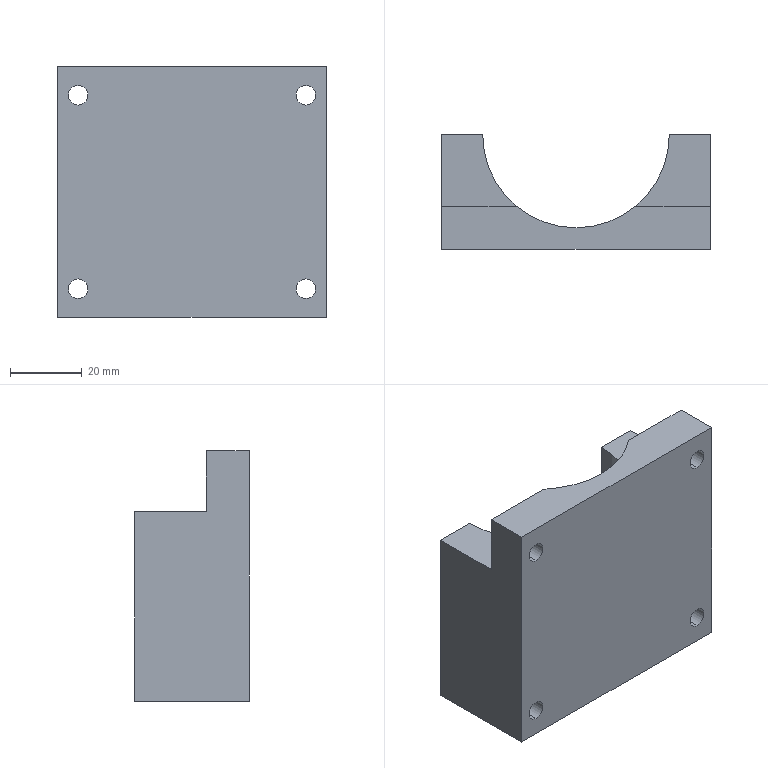Part | SolidWorks | features HoleWzd 2, ICE 2, Extrusion 1 | 1 solid | 48 faces | box 75 x 32 x 70 mm | volume 77130 mm3 | cylinder 25 | plane 15 | cone 8 | commonest cylinder face diameters 4.2 x8 5.5 x8 10 x8 52.1 x1
STEP:
#1=CARTESIAN_POINT('',(-31.75,3.6,18.9));
#2=VERTEX_POINT('',#1);
#3=CARTESIAN_POINT('',(-31.75,3.6,23.1));
#4=VERTEX_POINT('',#3);
#5=CARTESIAN_POINT('',(-31.75,3.6,21.));
#6=DIRECTION('',(0.,1.,0.));
#7=DIRECTION('',(0.,0.,1.));
#8=AXIS2_PLACEMENT_3D('',#5,#6,#7);
#9=CIRCLE('',#8,2.1);
#10=EDGE_CURVE('',#2,#4,#9,.T.);
#11=ORIENTED_EDGE('',*,*,#10,.F.);
#12=CARTESIAN_POINT('',(-31.75,16.,18.9));
#13=VERTEX_POINT('',#12);
#14=CARTESIAN_POINT('',(-31.75,16.,18.9));
#15=DIRECTION('',(0.,1.,0.));
#16=VECTOR('',#15,1000.);
#17=LINE('',#14,#16);
#18=EDGE_CURVE('',#2,#13,#17,.T.);
#19=ORIENTED_EDGE('',*,*,#18,.T.);
#20=CARTESIAN_POINT('',(-31.75,16.,23.1));
#21=VERTEX_POINT('',#20);
#22=CARTESIAN_POINT('',(-31.75,16.,21.));
#23=DIRECTION('',(0.,1.,0.));
#24=DIRECTION('',(0.,0.,1.));
#25=AXIS2_PLACEMENT_3D('',#22,#23,#24);
#26=CIRCLE('',#25,2.1);
#27=EDGE_CURVE('',#13,#21,#26,.T.);
#28=ORIENTED_EDGE('',*,*,#27,.T.);
#29=CARTESIAN_POINT('',(-31.75,16.,23.1));
#30=DIRECTION('',(0.,1.,0.));
#31=VECTOR('',#30,1000.);
#32=LINE('',#29,#31);
#33=EDGE_CURVE('',#4,#21,#32,.T.);
#34=ORIENTED_EDGE('',*,*,#33,.F.);
#35=EDGE_LOOP('',(#11,#19,#28,#34));
#36=FACE_OUTER_BOUND('',#35,.T.);
#37=CARTESIAN_POINT('',(-31.75,16.,21.));
#38=DIRECTION('',(0.,1.,0.));
#39=DIRECTION('',(0.,0.,1.));
#40=AXIS2_PLACEMENT_3D('',#37,#38,#39);
#41=CYLINDRICAL_SURFACE('',#40,2.1);
#42=ADVANCED_FACE('',(#36),#41,.F.);
#43=CARTESIAN_POINT('',(-31.75,2.338,21.));
#44=VERTEX_POINT('',#43);
#45=CARTESIAN_POINT('',(-31.75,3.6,23.1));
#46=DIRECTION('',(0.,0.515,0.8572));
#47=VECTOR('',#46,1000.);
#48=LINE('',#45,#47);
#49=EDGE_CURVE('',#44,#4,#48,.T.);
#50=ORIENTED_EDGE('',*,*,#49,.F.);
#51=CARTESIAN_POINT('',(-31.75,3.6,18.9));
#52=DIRECTION('',(0.,0.515,-0.8572));
#53=VECTOR('',#52,1000.);
#54=LINE('',#51,#53);
#55=EDGE_CURVE('',#44,#2,#54,.T.);
#56=ORIENTED_EDGE('',*,*,#55,.T.);
#57=ORIENTED_EDGE('',*,*,#10,.T.);
#58=EDGE_LOOP('',(#50,#56,#57));
#59=FACE_OUTER_BOUND('',#58,.T.);
#60=CARTESIAN_POINT('',(-31.75,3.6,21.));
#61=DIRECTION('',(0.,1.,0.));
#62=DIRECTION('',(0.,0.,1.));
#63=AXIS2_PLACEMENT_3D('',#60,#61,#62);
#64=CONICAL_SURFACE('',#63,2.1,1.03);
#65=ADVANCED_FACE('',(#59),#64,.F.);
#66=CARTESIAN_POINT('',(-31.75,3.6,42.9));
#67=VERTEX_POINT('',#66);
#68=CARTESIAN_POINT('',(-31.75,3.6,47.1));
#69=VERTEX_POINT('',#68);
#70=CARTESIAN_POINT('',(-31.75,3.6,45.));
#71=DIRECTION('',(0.,1.,0.));
#72=DIRECTION('',(0.,0.,1.));
#73=AXIS2_PLACEMENT_3D('',#70,#71,#72);
#74=CIRCLE('',#73,2.1);
#75=EDGE_CURVE('',#67,#69,#74,.T.);
#76=ORIENTED_EDGE('',*,*,#75,.F.);
#77=CARTESIAN_POINT('',(-31.75,16.,42.9));
#78=VERTEX_POINT('',#77);
#79=CARTESIAN_POINT('',(-31.75,16.,42.9));
#80=DIRECTION('',(0.,1.,0.));
#81=VECTOR('',#80,1000.);
#82=LINE('',#79,#81);
#83=EDGE_CURVE('',#67,#78,#82,.T.);
#84=ORIENTED_EDGE('',*,*,#83,.T.);
#85=CARTESIAN_POINT('',(-31.75,16.,47.1));
#86=VERTEX_POINT('',#85);
#87=CARTESIAN_POINT('',(-31.75,16.,45.));
#88=DIRECTION('',(0.,1.,0.));
#89=DIRECTION('',(0.,0.,1.));
#90=AXIS2_PLACEMENT_3D('',#87,#88,#89);
#91=CIRCLE('',#90,2.1);
#92=EDGE_CURVE('',#78,#86,#91,.T.);
#93=ORIENTED_EDGE('',*,*,#92,.T.);
#94=CARTESIAN_POINT('',(-31.75,16.,47.1));
#95=DIRECTION('',(0.,1.,0.));
#96=VECTOR('',#95,1000.);
#97=LINE('',#94,#96);
#98=EDGE_CURVE('',#69,#86,#97,.T.);
#99=ORIENTED_EDGE('',*,*,#98,.F.);
#100=EDGE_LOOP('',(#76,#84,#93,#99));
#101=FACE_OUTER_BOUND('',#100,.T.);
#102=CARTESIAN_POINT('',(-31.75,16.,45.));
#103=DIRECTION('',(0.,1.,0.));
#104=DIRECTION('',(0.,0.,1.));
#105=AXIS2_PLACEMENT_3D('',#102,#103,#104);
#106=CYLINDRICAL_SURFACE('',#105,2.1);
#107=ADVANCED_FACE('',(#101),#106,.F.);
#108=CARTESIAN_POINT('',(-31.75,2.338,45.));
#109=VERTEX_POINT('',#108);
#110=CARTESIAN_POINT('',(-31.75,3.6,47.1));
#111=DIRECTION('',(0.,0.515,0.8572));
#112=VECTOR('',#111,1000.);
#113=LINE('',#110,#112);
#114=EDGE_CURVE('',#109,#69,#113,.T.);
#115=ORIENTED_EDGE('',*,*,#114,.F.);
#116=CARTESIAN_POINT('',(-31.75,3.6,42.9));
#117=DIRECTION('',(0.,0.515,-0.8572));
#118=VECTOR('',#117,1000.);
#119=LINE('',#116,#118);
#120=EDGE_CURVE('',#109,#67,#119,.T.);
#121=ORIENTED_EDGE('',*,*,#120,.T.);
#122=ORIENTED_EDGE('',*,*,#75,.T.);
#123=EDGE_LOOP('',(#115,#121,#122));
#124=FACE_OUTER_BOUND('',#123,.T.);
#125=CARTESIAN_POINT('',(-31.75,3.6,45.));
#126=DIRECTION('',(0.,1.,0.));
#127=DIRECTION('',(0.,0.,1.));
#128=AXIS2_PLACEMENT_3D('',#125,#126,#127);
#129=CONICAL_SURFACE('',#128,2.1,1.03);
#130=ADVANCED_FACE('',(#124),#129,.F.);
#131=CARTESIAN_POINT('',(31.75,3.6,18.9));
#132=VERTEX_POINT('',#131);
#133=CARTESIAN_POINT('',(31.75,3.6,23.1));
#134=VERTEX_POINT('',#133);
#135=CARTESIAN_POINT('',(31.75,3.6,21.));
#136=DIRECTION('',(0.,1.,0.));
#137=DIRECTION('',(0.,0.,1.));
#138=AXIS2_PLACEMENT_3D('',#135,#136,#137);
#139=CIRCLE('',#138,2.1);
#140=EDGE_CURVE('',#132,#134,#139,.T.);
#141=ORIENTED_EDGE('',*,*,#140,.F.);
#142=CARTESIAN_POINT('',(31.75,16.,18.9));
#143=VERTEX_POINT('',#142);
#144=CARTESIAN_POINT('',(31.75,16.,18.9));
#145=DIRECTION('',(0.,1.,0.));
#146=VECTOR('',#145,1000.);
#147=LINE('',#144,#146);
#148=EDGE_CURVE('',#132,#143,#147,.T.);
#149=ORIENTED_EDGE('',*,*,#148,.T.);
#150=CARTESIAN_POINT('',(31.75,16.,23.1));
#151=VERTEX_POINT('',#150);
#152=CARTESIAN_POINT('',(31.75,16.,21.));
#153=DIRECTION('',(0.,1.,0.));
#154=DIRECTION('',(0.,0.,1.));
#155=AXIS2_PLACEMENT_3D('',#152,#153,#154);
#156=CIRCLE('',#155,2.1);
#157=EDGE_CURVE('',#143,#151,#156,.T.);
#158=ORIENTED_EDGE('',*,*,#157,.T.);
#159=CARTESIAN_POINT('',(31.75,16.,23.1));
#160=DIRECTION('',(0.,1.,0.));
#161=VECTOR('',#160,1000.);
#162=LINE('',#159,#161);
#163=EDGE_CURVE('',#134,#151,#162,.T.);
#164=ORIENTED_EDGE('',*,*,#163,.F.);
#165=EDGE_LOOP('',(#141,#149,#158,#164));
#166=FACE_OUTER_BOUND('',#165,.T.);
#167=CARTESIAN_POINT('',(31.75,16.,21.));
#168=DIRECTION('',(0.,1.,0.));
#169=DIRECTION('',(0.,0.,1.));
#170=AXIS2_PLACEMENT_3D('',#167,#168,#169);
#171=CYLINDRICAL_SURFACE('',#170,2.1);
#172=ADVANCED_FACE('',(#166),#171,.F.);
#173=CARTESIAN_POINT('',(31.75,2.338,21.));
#174=VERTEX_POINT('',#173);
#175=CARTESIAN_POINT('',(31.75,3.6,23.1));
#176=DIRECTION('',(0.,0.515,0.8572));
#177=VECTOR('',#176,1000.);
#178=LINE('',#175,#177);
#179=EDGE_CURVE('',#174,#134,#178,.T.);
#180=ORIENTED_EDGE('',*,*,#179,.F.);
#181=CARTESIAN_POINT('',(31.75,3.6,18.9));
#182=DIRECTION('',(0.,0.515,-0.8572));
#183=VECTOR('',#182,1000.);
#184=LINE('',#181,#183);
#185=EDGE_CURVE('',#174,#132,#184,.T.);
#186=ORIENTED_EDGE('',*,*,#185,.T.);
#187=ORIENTED_EDGE('',*,*,#140,.T.);
#188=EDGE_LOOP('',(#180,#186,#187));
#189=FACE_OUTER_BOUND('',#188,.T.);
#190=CARTESIAN_POINT('',(31.75,3.6,21.));
#191=DIRECTION('',(0.,1.,0.));
#192=DIRECTION('',(0.,0.,1.));
#193=AXIS2_PLACEMENT_3D('',#190,#191,#192);
#194=CONICAL_SURFACE('',#193,2.1,1.03);
#195=ADVANCED_FACE('',(#189),#194,.F.);
#196=CARTESIAN_POINT('',(31.75,3.6,42.9));
#197=VERTEX_POINT('',#196);
#198=CARTESIAN_POINT('',(31.75,3.6,47.1));
#199=VERTEX_POINT('',#198);
#200=CARTESIAN_POINT('',(31.75,3.6,45.));
#201=DIRECTION('',(0.,1.,0.));
#202=DIRECTION('',(0.,0.,1.));
#203=AXIS2_PLACEMENT_3D('',#200,#201,#202);
#204=CIRCLE('',#203,2.1);
#205=EDGE_CURVE('',#197,#199,#204,.T.);
#206=ORIENTED_EDGE('',*,*,#205,.F.);
#207=CARTESIAN_POINT('',(31.75,16.,42.9));
#208=VERTEX_POINT('',#207);
#209=CARTESIAN_POINT('',(31.75,16.,42.9));
#210=DIRECTION('',(0.,1.,0.));
#211=VECTOR('',#210,1000.);
#212=LINE('',#209,#211);
#213=EDGE_CURVE('',#197,#208,#212,.T.);
#214=ORIENTED_EDGE('',*,*,#213,.T.);
#215=CARTESIAN_POINT('',(31.75,16.,47.1));
#216=VERTEX_POINT('',#215);
#217=CARTESIAN_POINT('',(31.75,16.,45.));
#218=DIRECTION('',(0.,1.,0.));
#219=DIRECTION('',(0.,0.,1.));
#220=AXIS2_PLACEMENT_3D('',#217,#218,#219);
#221=CIRCLE('',#220,2.1);
#222=EDGE_CURVE('',#208,#216,#221,.T.);
#223=ORIENTED_EDGE('',*,*,#222,.T.);
#224=CARTESIAN_POINT('',(31.75,16.,47.1));
#225=DIRECTION('',(0.,1.,0.));
#226=VECTOR('',#225,1000.);
#227=LINE('',#224,#226);
#228=EDGE_CURVE('',#199,#216,#227,.T.);
#229=ORIENTED_EDGE('',*,*,#228,.F.);
#230=EDGE_LOOP('',(#206,#214,#223,#229));
#231=FACE_OUTER_BOUND('',#230,.T.);
#232=CARTESIAN_POINT('',(31.75,16.,45.));
#233=DIRECTION('',(0.,1.,0.));
#234=DIRECTION('',(0.,0.,1.));
#235=AXIS2_PLACEMENT_3D('',#232,#233,#234);
#236=CYLINDRICAL_SURFACE('',#235,2.1);
#237=ADVANCED_FACE('',(#231),#236,.F.);
#238=CARTESIAN_POINT('',(31.75,2.338,45.));
#239=VERTEX_POINT('',#238);
#240=CARTESIAN_POINT('',(31.75,3.6,47.1));
#241=DIRECTION('',(0.,0.515,0.8572));
#242=VECTOR('',#241,1000.);
#243=LINE('',#240,#242);
#244=EDGE_CURVE('',#239,#199,#243,.T.);
#245=ORIENTED_EDGE('',*,*,#244,.F.);
#246=CARTESIAN_POINT('',(31.75,3.6,42.9));
#247=DIRECTION('',(0.,0.515,-0.8572));
#248=VECTOR('',#247,1000.);
#249=LINE('',#246,#248);
#250=EDGE_CURVE('',#239,#197,#249,.T.);
#251=ORIENTED_EDGE('',*,*,#250,.T.);
#252=ORIENTED_EDGE('',*,*,#205,.T.);
#253=EDGE_LOOP('',(#245,#251,#252));
#254=FACE_OUTER_BOUND('',#253,.T.);
#255=CARTESIAN_POINT('',(31.75,3.6,45.));
#256=DIRECTION('',(0.,1.,0.));
#257=DIRECTION('',(0.,0.,1.));
#258=AXIS2_PLACEMENT_3D('',#255,#256,#257);
#259=CONICAL_SURFACE('',#258,2.1,1.03);
#260=ADVANCED_FACE('',(#254),#259,.F.);
#261=CARTESIAN_POINT('',(-31.775,-11.,3.));
#262=VERTEX_POINT('',#261);
#263=CARTESIAN_POINT('',(-31.775,-11.,13.));
#264=VERTEX_POINT('',#263);
#265=CARTESIAN_POINT('',(-31.775,-11.,8.));
#266=DIRECTION('',(0.,1.,0.));
#267=DIRECTION('',(0.,0.,1.));
#268=AXIS2_PLACEMENT_3D('',#265,#266,#267);
#269=CIRCLE('',#268,5.);
#270=EDGE_CURVE('',#262,#264,#269,.T.);
#271=ORIENTED_EDGE('',*,*,#270,.F.);
#272=CARTESIAN_POINT('',(-31.775,16.,3.));
#273=VERTEX_POINT('',#272);
#274=CARTESIAN_POINT('',(-31.775,16.,3.));
#275=DIRECTION('',(0.,1.,0.));
#276=VECTOR('',#275,1000.);
#277=LINE('',#274,#276);
#278=EDGE_CURVE('',#262,#273,#277,.T.);
#279=ORIENTED_EDGE('',*,*,#278,.T.);
#280=CARTESIAN_POINT('',(-31.775,16.,13.));
#281=VERTEX_POINT('',#280);
#282=CARTESIAN_POINT('',(-31.775,16.,8.));
#283=DIRECTION('',(0.,1.,0.));
#284=DIRECTION('',(0.,0.,1.));
#285=AXIS2_PLACEMENT_3D('',#282,#283,#284);
#286=CIRCLE('',#285,5.);
#287=EDGE_CURVE('',#273,#281,#286,.T.);
#288=ORIENTED_EDGE('',*,*,#287,.T.);
#289=CARTESIAN_POINT('',(-31.775,16.,13.));
#290=DIRECTION('',(0.,1.,0.));
#291=VECTOR('',#290,1000.);
#292=LINE('',#289,#291);
#293=EDGE_CURVE('',#264,#281,#292,.T.);
#294=ORIENTED_EDGE('',*,*,#293,.F.);
#295=EDGE_LOOP('',(#271,#279,#288,#294));
#296=FACE_OUTER_BOUND('',#295,.T.);
#297=CARTESIAN_POINT('',(-31.775,16.,8.));
#298=DIRECTION('',(0.,1.,0.));
#299=DIRECTION('',(0.,0.,1.));
#300=AXIS2_PLACEMENT_3D('',#297,#298,#299);
#301=CYLINDRICAL_SURFACE('',#300,5.);
#302=ADVANCED_FACE('',(#296),#301,.F.);
#303=CARTESIAN_POINT('',(-31.775,-16.,5.25));
#304=VERTEX_POINT('',#303);
#305=CARTESIAN_POINT('',(-31.775,-16.,10.75));
#306=VERTEX_POINT('',#305);
#307=CARTESIAN_POINT('',(-31.775,-16.,8.));
#308=DIRECTION('',(0.,1.,0.));
#309=DIRECTION('',(0.,0.,1.));
#310=AXIS2_PLACEMENT_3D('',#307,#308,#309);
#311=CIRCLE('',#310,2.75);
#312=EDGE_CURVE('',#304,#306,#311,.T.);
#313=ORIENTED_EDGE('',*,*,#312,.F.);
#314=CARTESIAN_POINT('',(-31.775,-11.,5.25));
#315=VERTEX_POINT('',#314);
#316=CARTESIAN_POINT('',(-31.775,16.,5.25));
#317=DIRECTION('',(0.,1.,0.));
#318=VECTOR('',#317,1000.);
#319=LINE('',#316,#318);
#320=EDGE_CURVE('',#304,#315,#319,.T.);
#321=ORIENTED_EDGE('',*,*,#320,.T.);
#322=CARTESIAN_POINT('',(-31.775,-11.,10.75));
#323=VERTEX_POINT('',#322);
#324=CARTESIAN_POINT('',(-31.775,-11.,8.));
#325=DIRECTION('',(0.,1.,0.));
#326=DIRECTION('',(0.,0.,1.));
#327=AXIS2_PLACEMENT_3D('',#324,#325,#326);
#328=CIRCLE('',#327,2.75);
#329=EDGE_CURVE('',#315,#323,#328,.T.);
#330=ORIENTED_EDGE('',*,*,#329,.T.);
#331=CARTESIAN_POINT('',(-31.775,16.,10.75));
#332=DIRECTION('',(0.,1.,0.));
#333=VECTOR('',#332,1000.);
#334=LINE('',#331,#333);
#335=EDGE_CURVE('',#306,#323,#334,.T.);
#336=ORIENTED_EDGE('',*,*,#335,.F.);
#337=EDGE_LOOP('',(#313,#321,#330,#336));
#338=FACE_OUTER_BOUND('',#337,.T.);
#339=CARTESIAN_POINT('',(-31.775,16.,8.));
#340=DIRECTION('',(0.,1.,0.));
#341=DIRECTION('',(0.,0.,1.));
#342=AXIS2_PLACEMENT_3D('',#339,#340,#341);
#343=CYLINDRICAL_SURFACE('',#342,2.75);
#344=ADVANCED_FACE('',(#338),#343,.F.);
#345=CARTESIAN_POINT('',(-31.775,-11.,57.));
#346=VERTEX_POINT('',#345);
#347=CARTESIAN_POINT('',(-31.775,-11.,67.));
#348=VERTEX_POINT('',#347);
#349=CARTESIAN_POINT('',(-31.775,-11.,62.));
#350=DIRECTION('',(0.,1.,0.));
#351=DIRECTION('',(0.,0.,1.));
#352=AXIS2_PLACEMENT_3D('',#349,#350,#351);
#353=CIRCLE('',#352,5.);
#354=EDGE_CURVE('',#346,#348,#353,.T.);
#355=ORIENTED_EDGE('',*,*,#354,.F.);
#356=CARTESIAN_POINT('',(-31.775,-4.,57.));
#357=VERTEX_POINT('',#356);
#358=CARTESIAN_POINT('',(-31.775,16.,57.));
#359=DIRECTION('',(0.,1.,0.));
#360=VECTOR('',#359,1000.);
#361=LINE('',#358,#360);
#362=EDGE_CURVE('',#346,#357,#361,.T.);
#363=ORIENTED_EDGE('',*,*,#362,.T.);
#364=CARTESIAN_POINT('',(-31.775,-4.,67.));
#365=VERTEX_POINT('',#364);
#366=CARTESIAN_POINT('',(-31.775,-4.,62.));
#367=DIRECTION('',(0.,1.,0.));
#368=DIRECTION('',(0.,0.,-1.));
#369=AXIS2_PLACEMENT_3D('',#366,#367,#368);
#370=CIRCLE('',#369,5.);
#371=EDGE_CURVE('',#357,#365,#370,.T.);
#372=ORIENTED_EDGE('',*,*,#371,.T.);
#373=CARTESIAN_POINT('',(-31.775,16.,67.));
#374=DIRECTION('',(0.,1.,0.));
#375=VECTOR('',#374,1000.);
#376=LINE('',#373,#375);
#377=EDGE_CURVE('',#348,#365,#376,.T.);
#378=ORIENTED_EDGE('',*,*,#377,.F.);
#379=EDGE_LOOP('',(#355,#363,#372,#378));
#380=FACE_OUTER_BOUND('',#379,.T.);
#381=CARTESIAN_POINT('',(-31.775,16.,62.));
#382=DIRECTION('',(0.,1.,0.));
#383=DIRECTION('',(0.,0.,1.));
#384=AXIS2_PLACEMENT_3D('',#381,#382,#383);
#385=CYLINDRICAL_SURFACE('',#384,5.);
#386=ADVANCED_FACE('',(#380),#385,.F.);
#387=CARTESIAN_POINT('',(-31.775,-16.,59.25));
#388=VERTEX_POINT('',#387);
#389=CARTESIAN_POINT('',(-31.775,-16.,64.75));
#390=VERTEX_POINT('',#389);
#391=CARTESIAN_POINT('',(-31.775,-16.,62.));
#392=DIRECTION('',(0.,1.,0.));
#393=DIRECTION('',(0.,0.,1.));
#394=AXIS2_PLACEMENT_3D('',#391,#392,#393);
#395=CIRCLE('',#394,2.75);
#396=EDGE_CURVE('',#388,#390,#395,.T.);
#397=ORIENTED_EDGE('',*,*,#396,.F.);
#398=CARTESIAN_POINT('',(-31.775,-11.,59.25));
#399=VERTEX_POINT('',#398);
#400=CARTESIAN_POINT('',(-31.775,16.,59.25));
#401=DIRECTION('',(0.,1.,0.));
#402=VECTOR('',#401,1000.);
#403=LINE('',#400,#402);
#404=EDGE_CURVE('',#388,#399,#403,.T.);
#405=ORIENTED_EDGE('',*,*,#404,.T.);
#406=CARTESIAN_POINT('',(-31.775,-11.,64.75));
#407=VERTEX_POINT('',#406);
#408=CARTESIAN_POINT('',(-31.775,-11.,62.));
#409=DIRECTION('',(0.,1.,0.));
#410=DIRECTION('',(0.,0.,1.));
#411=AXIS2_PLACEMENT_3D('',#408,#409,#410);
#412=CIRCLE('',#411,2.75);
#413=EDGE_CURVE('',#399,#407,#412,.T.);
#414=ORIENTED_EDGE('',*,*,#413,.T.);
#415=CARTESIAN_POINT('',(-31.775,16.,64.75));
#416=DIRECTION('',(0.,1.,0.));
#417=VECTOR('',#416,1000.);
#418=LINE('',#415,#417);
#419=EDGE_CURVE('',#390,#407,#418,.T.);
#420=ORIENTED_EDGE('',*,*,#419,.F.);
#421=EDGE_LOOP('',(#397,#405,#414,#420));
#422=FACE_OUTER_BOUND('',#421,.T.);
#423=CARTESIAN_POINT('',(-31.775,16.,62.));
#424=DIRECTION('',(0.,1.,0.));
#425=DIRECTION('',(0.,0.,1.));
#426=AXIS2_PLACEMENT_3D('',#423,#424,#425);
#427=CYLINDRICAL_SURFACE('',#426,2.75);
#428=ADVANCED_FACE('',(#422),#427,.F.);
#429=CARTESIAN_POINT('',(31.775,-11.,57.));
#430=VERTEX_POINT('',#429);
#431=CARTESIAN_POINT('',(31.775,-11.,67.));
#432=VERTEX_POINT('',#431);
#433=CARTESIAN_POINT('',(31.775,-11.,62.));
#434=DIRECTION('',(0.,1.,0.));
#435=DIRECTION('',(0.,0.,1.));
#436=AXIS2_PLACEMENT_3D('',#433,#434,#435);
#437=CIRCLE('',#436,5.);
#438=EDGE_CURVE('',#430,#432,#437,.T.);
#439=ORIENTED_EDGE('',*,*,#438,.F.);
#440=CARTESIAN_POINT('',(31.775,-4.,57.));
#441=VERTEX_POINT('',#440);
#442=CARTESIAN_POINT('',(31.775,16.,57.));
#443=DIRECTION('',(0.,1.,0.));
#444=VECTOR('',#443,1000.);
#445=LINE('',#442,#444);
#446=EDGE_CURVE('',#430,#441,#445,.T.);
#447=ORIENTED_EDGE('',*,*,#446,.T.);
#448=CARTESIAN_POINT('',(31.775,-4.,67.));
#449=VERTEX_POINT('',#448);
#450=CARTESIAN_POINT('',(31.775,-4.,62.));
#451=DIRECTION('',(0.,1.,0.));
#452=DIRECTION('',(0.,0.,-1.));
#453=AXIS2_PLACEMENT_3D('',#450,#451,#452);
#454=CIRCLE('',#453,5.);
#455=EDGE_CURVE('',#441,#449,#454,.T.);
#456=ORIENTED_EDGE('',*,*,#455,.T.);
#457=CARTESIAN_POINT('',(31.775,16.,67.));
#458=DIRECTION('',(0.,1.,0.));
#459=VECTOR('',#458,1000.);
#460=LINE('',#457,#459);
#461=EDGE_CURVE('',#432,#449,#460,.T.);
#462=ORIENTED_EDGE('',*,*,#461,.F.);
#463=EDGE_LOOP('',(#439,#447,#456,#462));
#464=FACE_OUTER_BOUND('',#463,.T.);
#465=CARTESIAN_POINT('',(31.775,16.,62.));
#466=DIRECTION('',(0.,1.,0.));
#467=DIRECTION('',(0.,0.,1.));
#468=AXIS2_PLACEMENT_3D('',#465,#466,#467);
#469=CYLINDRICAL_SURFACE('',#468,5.);
#470=ADVANCED_FACE('',(#464),#469,.F.);
#471=CARTESIAN_POINT('',(31.775,-16.,59.25));
#472=VERTEX_POINT('',#471);
#473=CARTESIAN_POINT('',(31.775,-16.,64.75));
#474=VERTEX_POINT('',#473);
#475=CARTESIAN_POINT('',(31.775,-16.,62.));
#476=DIRECTION('',(0.,1.,0.));
#477=DIRECTION('',(0.,0.,1.));
#478=AXIS2_PLACEMENT_3D('',#475,#476,#477);
#479=CIRCLE('',#478,2.75);
#480=EDGE_CURVE('',#472,#474,#479,.T.);
#481=ORIENTED_EDGE('',*,*,#480,.F.);
#482=CARTESIAN_POINT('',(31.775,-11.,59.25));
#483=VERTEX_POINT('',#482);
#484=CARTESIAN_POINT('',(31.775,16.,59.25));
#485=DIRECTION('',(0.,1.,0.));
#486=VECTOR('',#485,1000.);
#487=LINE('',#484,#486);
#488=EDGE_CURVE('',#472,#483,#487,.T.);
#489=ORIENTED_EDGE('',*,*,#488,.T.);
#490=CARTESIAN_POINT('',(31.775,-11.,64.75));
#491=VERTEX_POINT('',#490);
#492=CARTESIAN_POINT('',(31.775,-11.,62.));
#493=DIRECTION('',(0.,1.,0.));
#494=DIRECTION('',(0.,0.,1.));
#495=AXIS2_PLACEMENT_3D('',#492,#493,#494);
#496=CIRCLE('',#495,2.75);
#497=EDGE_CURVE('',#483,#491,#496,.T.);
#498=ORIENTED_EDGE('',*,*,#497,.T.);
#499=CARTESIAN_POINT('',(31.775,16.,64.75));
#500=DIRECTION('',(0.,1.,0.));
#501=VECTOR('',#500,1000.);
#502=LINE('',#499,#501);
#503=EDGE_CURVE('',#474,#491,#502,.T.);
#504=ORIENTED_EDGE('',*,*,#503,.F.);
#505=EDGE_LOOP('',(#481,#489,#498,#504));
#506=FACE_OUTER_BOUND('',#505,.T.);
#507=CARTESIAN_POINT('',(31.775,16.,62.));
#508=DIRECTION('',(0.,1.,0.));
#509=DIRECTION('',(0.,0.,1.));
#510=AXIS2_PLACEMENT_3D('',#507,#508,#509);
#511=CYLINDRICAL_SURFACE('',#510,2.75);
#512=ADVANCED_FACE('',(#506),#511,.F.);
#513=CARTESIAN_POINT('',(31.775,-11.,3.));
#514=VERTEX_POINT('',#513);
#515=CARTESIAN_POINT('',(31.775,-11.,13.));
#516=VERTEX_POINT('',#515);
#517=CARTESIAN_POINT('',(31.775,-11.,8.));
#518=DIRECTION('',(0.,1.,0.));
#519=DIRECTION('',(0.,0.,1.));
#520=AXIS2_PLACEMENT_3D('',#517,#518,#519);
#521=CIRCLE('',#520,5.);
#522=EDGE_CURVE('',#514,#516,#521,.T.);
#523=ORIENTED_EDGE('',*,*,#522,.F.);
#524=CARTESIAN_POINT('',(31.775,16.,3.));
#525=VERTEX_POINT('',#524);
#526=CARTESIAN_POINT('',(31.775,16.,3.));
#527=DIRECTION('',(0.,1.,0.));
#528=VECTOR('',#527,1000.);
#529=LINE('',#526,#528);
#530=EDGE_CURVE('',#514,#525,#529,.T.);
#531=ORIENTED_EDGE('',*,*,#530,.T.);
#532=CARTESIAN_POINT('',(31.775,16.,13.));
#533=VERTEX_POINT('',#532);
#534=CARTESIAN_POINT('',(31.775,16.,8.));
#535=DIRECTION('',(0.,1.,0.));
#536=DIRECTION('',(0.,0.,1.));
#537=AXIS2_PLACEMENT_3D('',#534,#535,#536);
#538=CIRCLE('',#537,5.);
#539=EDGE_CURVE('',#525,#533,#538,.T.);
#540=ORIENTED_EDGE('',*,*,#539,.T.);
#541=CARTESIAN_POINT('',(31.775,16.,13.));
#542=DIRECTION('',(0.,1.,0.));
#543=VECTOR('',#542,1000.);
#544=LINE('',#541,#543);
#545=EDGE_CURVE('',#516,#533,#544,.T.);
#546=ORIENTED_EDGE('',*,*,#545,.F.);
#547=EDGE_LOOP('',(#523,#531,#540,#546));
#548=FACE_OUTER_BOUND('',#547,.T.);
#549=CARTESIAN_POINT('',(31.775,16.,8.));
#550=DIRECTION('',(0.,1.,0.));
#551=DIRECTION('',(0.,0.,1.));
#552=AXIS2_PLACEMENT_3D('',#549,#550,#551);
#553=CYLINDRICAL_SURFACE('',#552,5.);
#554=ADVANCED_FACE('',(#548),#553,.F.);
#555=CARTESIAN_POINT('',(31.775,-16.,5.25));
#556=VERTEX_POINT('',#555);
#557=CARTESIAN_POINT('',(31.775,-16.,10.75));
#558=VERTEX_POINT('',#557);
#559=CARTESIAN_POINT('',(31.775,-16.,8.));
#560=DIRECTION('',(0.,1.,0.));
#561=DIRECTION('',(0.,0.,1.));
#562=AXIS2_PLACEMENT_3D('',#559,#560,#561);
#563=CIRCLE('',#562,2.75);
#564=EDGE_CURVE('',#556,#558,#563,.T.);
#565=ORIENTED_EDGE('',*,*,#564,.F.);
#566=CARTESIAN_POINT('',(31.775,-11.,5.25));
#567=VERTEX_POINT('',#566);
#568=CARTESIAN_POINT('',(31.775,16.,5.25));
#569=DIRECTION('',(0.,1.,0.));
#570=VECTOR('',#569,1000.);
#571=LINE('',#568,#570);
#572=EDGE_CURVE('',#556,#567,#571,.T.);
#573=ORIENTED_EDGE('',*,*,#572,.T.);
#574=CARTESIAN_POINT('',(31.775,-11.,10.75));
#575=VERTEX_POINT('',#574);
#576=CARTESIAN_POINT('',(31.775,-11.,8.));
#577=DIRECTION('',(0.,1.,0.));
#578=DIRECTION('',(0.,0.,1.));
#579=AXIS2_PLACEMENT_3D('',#576,#577,#578);
#580=CIRCLE('',#579,2.75);
#581=EDGE_CURVE('',#567,#575,#580,.T.);
#582=ORIENTED_EDGE('',*,*,#581,.T.);
#583=CARTESIAN_POINT('',(31.775,16.,10.75));
#584=DIRECTION('',(0.,1.,0.));
#585=VECTOR('',#584,1000.);
#586=LINE('',#583,#585);
#587=EDGE_CURVE('',#558,#575,#586,.T.);
#588=ORIENTED_EDGE('',*,*,#587,.F.);
#589=EDGE_LOOP('',(#565,#573,#582,#588));
#590=FACE_OUTER_BOUND('',#589,.T.);
#591=CARTESIAN_POINT('',(31.775,16.,8.));
#592=DIRECTION('',(0.,1.,0.));
#593=DIRECTION('',(0.,0.,1.));
#594=AXIS2_PLACEMENT_3D('',#591,#592,#593);
#595=CYLINDRICAL_SURFACE('',#594,2.75);
#596=ADVANCED_FACE('',(#590),#595,.F.);
#597=CARTESIAN_POINT('',(31.75,16.,21.));
#598=DIRECTION('',(0.,1.,0.));
#599=DIRECTION('',(0.,0.,1.));
#600=AXIS2_PLACEMENT_3D('',#597,#598,#599);
#601=CIRCLE('',#600,2.1);
#602=EDGE_CURVE('',#151,#143,#601,.T.);
#603=ORIENTED_EDGE('',*,*,#602,.F.);
#604=ORIENTED_EDGE('',*,*,#157,.F.);
#605=EDGE_LOOP('',(#603,#604));
#606=FACE_BOUND('',#605,.T.);
#607=CARTESIAN_POINT('',(31.75,16.,45.));
#608=DIRECTION('',(0.,1.,0.));
#609=DIRECTION('',(0.,0.,1.));
#610=AXIS2_PLACEMENT_3D('',#607,#608,#609);
#611=CIRCLE('',#610,2.1);
#612=EDGE_CURVE('',#216,#208,#611,.T.);
#613=ORIENTED_EDGE('',*,*,#612,.F.);
#614=ORIENTED_EDGE('',*,*,#222,.F.);
#615=EDGE_LOOP('',(#613,#614));
#616=FACE_BOUND('',#615,.T.);
#617=CARTESIAN_POINT('',(31.775,16.,8.));
#618=DIRECTION('',(0.,1.,0.));
#619=DIRECTION('',(0.,0.,1.));
#620=AXIS2_PLACEMENT_3D('',#617,#618,#619);
#621=CIRCLE('',#620,5.);
#622=EDGE_CURVE('',#533,#525,#621,.T.);
#623=ORIENTED_EDGE('',*,*,#622,.F.);
#624=ORIENTED_EDGE('',*,*,#539,.F.);
#625=EDGE_LOOP('',(#623,#624));
#626=FACE_BOUND('',#625,.T.);
#627=CARTESIAN_POINT('',(26.05,16.,0.));
#628=VERTEX_POINT('',#627);
#629=CARTESIAN_POINT('',(26.05,16.,53.));
#630=VERTEX_POINT('',#629);
#631=CARTESIAN_POINT('',(26.05,16.,0.));
#632=DIRECTION('',(0.,0.,1.));
#633=VECTOR('',#632,1000.);
#634=LINE('',#631,#633);
#635=EDGE_CURVE('',#628,#630,#634,.T.);
#636=ORIENTED_EDGE('',*,*,#635,.T.);
#637=CARTESIAN_POINT('',(37.5,16.,53.));
#638=VERTEX_POINT('',#637);
#639=CARTESIAN_POINT('',(37.5,16.,53.));
#640=DIRECTION('',(-1.,0.,0.));
#641=VECTOR('',#640,1000.);
#642=LINE('',#639,#641);
#643=EDGE_CURVE('',#638,#630,#642,.T.);
#644=ORIENTED_EDGE('',*,*,#643,.F.);
#645=CARTESIAN_POINT('',(37.5,16.,0.));
#646=VERTEX_POINT('',#645);
#647=CARTESIAN_POINT('',(37.5,16.,70.));
#648=DIRECTION('',(0.,0.,-1.));
#649=VECTOR('',#648,1000.);
#650=LINE('',#647,#649);
#651=EDGE_CURVE('',#638,#646,#650,.T.);
#652=ORIENTED_EDGE('',*,*,#651,.T.);
#653=CARTESIAN_POINT('',(-37.5,16.,0.));
#654=DIRECTION('',(-1.,0.,0.));
#655=VECTOR('',#654,1000.);
#656=LINE('',#653,#655);
#657=EDGE_CURVE('',#646,#628,#656,.T.);
#658=ORIENTED_EDGE('',*,*,#657,.T.);
#659=EDGE_LOOP('',(#636,#644,#652,#658));
#660=FACE_OUTER_BOUND('',#659,.T.);
#661=CARTESIAN_POINT('',(-37.5,16.,70.));
#662=DIRECTION('',(0.,-1.,0.));
#663=DIRECTION('',(0.,0.,-1.));
#664=AXIS2_PLACEMENT_3D('',#661,#662,#663);
#665=PLANE('',#664);
#666=ADVANCED_FACE('',(#606,#616,#626,#660),#665,.F.);
#667=ORIENTED_EDGE('',*,*,#651,.F.);
#668=CARTESIAN_POINT('',(37.5,-4.,53.));
#669=VERTEX_POINT('',#668);
#670=CARTESIAN_POINT('',(37.5,16.,53.));
#671=DIRECTION('',(0.,-1.,0.));
#672=VECTOR('',#671,1000.);
#673=LINE('',#670,#672);
#674=EDGE_CURVE('',#638,#669,#673,.T.);
#675=ORIENTED_EDGE('',*,*,#674,.T.);
#676=CARTESIAN_POINT('',(37.5,-4.,70.));
#677=VERTEX_POINT('',#676);
#678=CARTESIAN_POINT('',(37.5,-4.,53.));
#679=DIRECTION('',(0.,0.,1.));
#680=VECTOR('',#679,1000.);
#681=LINE('',#678,#680);
#682=EDGE_CURVE('',#669,#677,#681,.T.);
#683=ORIENTED_EDGE('',*,*,#682,.T.);
#684=CARTESIAN_POINT('',(37.5,-16.,70.));
#685=VERTEX_POINT('',#684);
#686=CARTESIAN_POINT('',(37.5,-16.,70.));
#687=DIRECTION('',(0.,1.,0.));
#688=VECTOR('',#687,1000.);
#689=LINE('',#686,#688);
#690=EDGE_CURVE('',#685,#677,#689,.T.);
#691=ORIENTED_EDGE('',*,*,#690,.F.);
#692=CARTESIAN_POINT('',(37.5,-16.,0.));
#693=VERTEX_POINT('',#692);
#694=CARTESIAN_POINT('',(37.5,-16.,70.));
#695=DIRECTION('',(0.,0.,-1.));
#696=VECTOR('',#695,1000.);
#697=LINE('',#694,#696);
#698=EDGE_CURVE('',#685,#693,#697,.T.);
#699=ORIENTED_EDGE('',*,*,#698,.T.);
#700=CARTESIAN_POINT('',(37.5,-16.,0.));
#701=DIRECTION('',(0.,1.,0.));
#702=VECTOR('',#701,1000.);
#703=LINE('',#700,#702);
#704=EDGE_CURVE('',#693,#646,#703,.T.);
#705=ORIENTED_EDGE('',*,*,#704,.T.);
#706=EDGE_LOOP('',(#667,#675,#683,#691,#699,#705));
#707=FACE_OUTER_BOUND('',#706,.T.);
#708=CARTESIAN_POINT('',(37.5,-16.,70.));
#709=DIRECTION('',(-1.,0.,0.));
#710=DIRECTION('',(0.,0.,1.));
#711=AXIS2_PLACEMENT_3D('',#708,#709,#710);
#712=PLANE('',#711);
#713=ADVANCED_FACE('',(#707),#712,.F.);
#714=CARTESIAN_POINT('',(-31.75,16.,21.));
#715=DIRECTION('',(0.,1.,0.));
#716=DIRECTION('',(0.,0.,1.));
#717=AXIS2_PLACEMENT_3D('',#714,#715,#716);
#718=CIRCLE('',#717,2.1);
#719=EDGE_CURVE('',#21,#13,#718,.T.);
#720=ORIENTED_EDGE('',*,*,#719,.F.);
#721=ORIENTED_EDGE('',*,*,#27,.F.);
#722=EDGE_LOOP('',(#720,#721));
#723=FACE_BOUND('',#722,.T.);
#724=CARTESIAN_POINT('',(-31.75,16.,45.));
#725=DIRECTION('',(0.,1.,0.));
#726=DIRECTION('',(0.,0.,1.));
#727=AXIS2_PLACEMENT_3D('',#724,#725,#726);
#728=CIRCLE('',#727,2.1);
#729=EDGE_CURVE('',#86,#78,#728,.T.);
#730=ORIENTED_EDGE('',*,*,#729,.F.);
#731=ORIENTED_EDGE('',*,*,#92,.F.);
#732=EDGE_LOOP('',(#730,#731));
#733=FACE_BOUND('',#732,.T.);
#734=CARTESIAN_POINT('',(-31.775,16.,8.));
#735=DIRECTION('',(0.,1.,0.));
#736=DIRECTION('',(0.,0.,1.));
#737=AXIS2_PLACEMENT_3D('',#734,#735,#736);
#738=CIRCLE('',#737,5.);
#739=EDGE_CURVE('',#281,#273,#738,.T.);
#740=ORIENTED_EDGE('',*,*,#739,.F.);
#741=ORIENTED_EDGE('',*,*,#287,.F.);
#742=EDGE_LOOP('',(#740,#741));
#743=FACE_BOUND('',#742,.T.);
#744=CARTESIAN_POINT('',(-37.5,16.,53.));
#745=VERTEX_POINT('',#744);
#746=CARTESIAN_POINT('',(-37.5,16.,0.));
#747=VERTEX_POINT('',#746);
#748=CARTESIAN_POINT('',(-37.5,16.,70.));
#749=DIRECTION('',(0.,0.,-1.));
#750=VECTOR('',#749,1000.);
#751=LINE('',#748,#750);
#752=EDGE_CURVE('',#745,#747,#751,.T.);
#753=ORIENTED_EDGE('',*,*,#752,.F.);
#754=CARTESIAN_POINT('',(-26.05,16.,53.));
#755=VERTEX_POINT('',#754);
#756=CARTESIAN_POINT('',(37.5,16.,53.));
#757=DIRECTION('',(-1.,0.,0.));
#758=VECTOR('',#757,1000.);
#759=LINE('',#756,#758);
#760=EDGE_CURVE('',#755,#745,#759,.T.);
#761=ORIENTED_EDGE('',*,*,#760,.F.);
#762=CARTESIAN_POINT('',(-26.05,16.,0.));
#763=VERTEX_POINT('',#762);
#764=CARTESIAN_POINT('',(-26.05,16.,0.));
#765=DIRECTION('',(0.,0.,-1.));
#766=VECTOR('',#765,1000.);
#767=LINE('',#764,#766);
#768=EDGE_CURVE('',#755,#763,#767,.T.);
#769=ORIENTED_EDGE('',*,*,#768,.T.);
#770=CARTESIAN_POINT('',(-37.5,16.,0.));
#771=DIRECTION('',(-1.,0.,0.));
#772=VECTOR('',#771,1000.);
#773=LINE('',#770,#772);
#774=EDGE_CURVE('',#763,#747,#773,.T.);
#775=ORIENTED_EDGE('',*,*,#774,.T.);
#776=EDGE_LOOP('',(#753,#761,#769,#775));
#777=FACE_OUTER_BOUND('',#776,.T.);
#778=CARTESIAN_POINT('',(-37.5,16.,70.));
#779=DIRECTION('',(0.,-1.,0.));
#780=DIRECTION('',(0.,0.,-1.));
#781=AXIS2_PLACEMENT_3D('',#778,#779,#780);
#782=PLANE('',#781);
#783=ADVANCED_FACE('',(#723,#733,#743,#777),#782,.F.);
#784=CARTESIAN_POINT('',(-37.5,-4.,53.));
#785=VERTEX_POINT('',#784);
#786=CARTESIAN_POINT('',(-37.5,-4.,70.));
#787=VERTEX_POINT('',#786);
#788=CARTESIAN_POINT('',(-37.5,-4.,53.));
#789=DIRECTION('',(0.,0.,1.));
#790=VECTOR('',#789,1000.);
#791=LINE('',#788,#790);
#792=EDGE_CURVE('',#785,#787,#791,.T.);
#793=ORIENTED_EDGE('',*,*,#792,.F.);
#794=CARTESIAN_POINT('',(-37.5,16.,53.));
#795=DIRECTION('',(0.,-1.,0.));
#796=VECTOR('',#795,1000.);
#797=LINE('',#794,#796);
#798=EDGE_CURVE('',#745,#785,#797,.T.);
#799=ORIENTED_EDGE('',*,*,#798,.F.);
#800=ORIENTED_EDGE('',*,*,#752,.T.);
#801=CARTESIAN_POINT('',(-37.5,-16.,0.));
#802=VERTEX_POINT('',#801);
#803=CARTESIAN_POINT('',(-37.5,-16.,0.));
#804=DIRECTION('',(0.,-1.,0.));
#805=VECTOR('',#804,1000.);
#806=LINE('',#803,#805);
#807=EDGE_CURVE('',#747,#802,#806,.T.);
#808=ORIENTED_EDGE('',*,*,#807,.T.);
#809=CARTESIAN_POINT('',(-37.5,-16.,70.));
#810=VERTEX_POINT('',#809);
#811=CARTESIAN_POINT('',(-37.5,-16.,70.));
#812=DIRECTION('',(0.,0.,-1.));
#813=VECTOR('',#812,1000.);
#814=LINE('',#811,#813);
#815=EDGE_CURVE('',#810,#802,#814,.T.);
#816=ORIENTED_EDGE('',*,*,#815,.F.);
#817=CARTESIAN_POINT('',(-37.5,-16.,70.));
#818=DIRECTION('',(0.,-1.,0.));
#819=VECTOR('',#818,1000.);
#820=LINE('',#817,#819);
#821=EDGE_CURVE('',#787,#810,#820,.T.);
#822=ORIENTED_EDGE('',*,*,#821,.F.);
#823=EDGE_LOOP('',(#793,#799,#800,#808,#816,#822));
#824=FACE_OUTER_BOUND('',#823,.T.);
#825=CARTESIAN_POINT('',(-37.5,-16.,70.));
#826=DIRECTION('',(1.,0.,0.));
#827=DIRECTION('',(0.,0.,-1.));
#828=AXIS2_PLACEMENT_3D('',#825,#826,#827);
#829=PLANE('',#828);
#830=ADVANCED_FACE('',(#824),#829,.F.);
#831=CARTESIAN_POINT('',(-31.775,-16.,8.));
#832=DIRECTION('',(0.,1.,0.));
#833=DIRECTION('',(0.,0.,1.));
#834=AXIS2_PLACEMENT_3D('',#831,#832,#833);
#835=CIRCLE('',#834,2.75);
#836=EDGE_CURVE('',#306,#304,#835,.T.);
#837=ORIENTED_EDGE('',*,*,#836,.T.);
#838=ORIENTED_EDGE('',*,*,#312,.T.);
#839=EDGE_LOOP('',(#837,#838));
#840=FACE_BOUND('',#839,.T.);
#841=CARTESIAN_POINT('',(-31.775,-16.,62.));
#842=DIRECTION('',(0.,1.,0.));
#843=DIRECTION('',(0.,0.,1.));
#844=AXIS2_PLACEMENT_3D('',#841,#842,#843);
#845=CIRCLE('',#844,2.75);
#846=EDGE_CURVE('',#390,#388,#845,.T.);
#847=ORIENTED_EDGE('',*,*,#846,.T.);
#848=ORIENTED_EDGE('',*,*,#396,.T.);
#849=EDGE_LOOP('',(#847,#848));
#850=FACE_BOUND('',#849,.T.);
#851=CARTESIAN_POINT('',(31.775,-16.,62.));
#852=DIRECTION('',(0.,1.,0.));
#853=DIRECTION('',(0.,0.,1.));
#854=AXIS2_PLACEMENT_3D('',#851,#852,#853);
#855=CIRCLE('',#854,2.75);
#856=EDGE_CURVE('',#474,#472,#855,.T.);
#857=ORIENTED_EDGE('',*,*,#856,.T.);
#858=ORIENTED_EDGE('',*,*,#480,.T.);
#859=EDGE_LOOP('',(#857,#858));
#860=FACE_BOUND('',#859,.T.);
#861=CARTESIAN_POINT('',(31.775,-16.,8.));
#862=DIRECTION('',(0.,1.,0.));
#863=DIRECTION('',(0.,0.,1.));
#864=AXIS2_PLACEMENT_3D('',#861,#862,#863);
#865=CIRCLE('',#864,2.75);
#866=EDGE_CURVE('',#558,#556,#865,.T.);
#867=ORIENTED_EDGE('',*,*,#866,.T.);
#868=ORIENTED_EDGE('',*,*,#564,.T.);
#869=EDGE_LOOP('',(#867,#868));
#870=FACE_BOUND('',#869,.T.);
#871=CARTESIAN_POINT('',(-37.5,-16.,0.));
#872=DIRECTION('',(1.,0.,0.));
#873=VECTOR('',#872,1000.);
#874=LINE('',#871,#873);
#875=EDGE_CURVE('',#802,#693,#874,.T.);
#876=ORIENTED_EDGE('',*,*,#875,.T.);
#877=ORIENTED_EDGE('',*,*,#698,.F.);
#878=CARTESIAN_POINT('',(-37.5,-16.,70.));
#879=DIRECTION('',(1.,0.,0.));
#880=VECTOR('',#879,1000.);
#881=LINE('',#878,#880);
#882=EDGE_CURVE('',#810,#685,#881,.T.);
#883=ORIENTED_EDGE('',*,*,#882,.F.);
#884=ORIENTED_EDGE('',*,*,#815,.T.);
#885=EDGE_LOOP('',(#876,#877,#883,#884));
#886=FACE_OUTER_BOUND('',#885,.T.);
#887=CARTESIAN_POINT('',(-37.5,-16.,70.));
#888=DIRECTION('',(0.,1.,0.));
#889=DIRECTION('',(0.,0.,1.));
#890=AXIS2_PLACEMENT_3D('',#887,#888,#889);
#891=PLANE('',#890);
#892=ADVANCED_FACE('',(#840,#850,#860,#870,#886),#891,.F.);
#893=ORIENTED_EDGE('',*,*,#690,.T.);
#894=CARTESIAN_POINT('',(16.691,-4.,70.));
#895=VERTEX_POINT('',#894);
#896=CARTESIAN_POINT('',(37.5,-4.,70.));
#897=DIRECTION('',(-1.,0.,0.));
#898=VECTOR('',#897,1000.);
#899=LINE('',#896,#898);
#900=EDGE_CURVE('',#677,#895,#899,.T.);
#901=ORIENTED_EDGE('',*,*,#900,.T.);
#902=CARTESIAN_POINT('',(-16.691,-4.,70.));
#903=VERTEX_POINT('',#902);
#904=CARTESIAN_POINT('',(0.,16.,70.));
#905=DIRECTION('',(0.,0.,1.));
#906=DIRECTION('',(1.,0.,0.));
#907=AXIS2_PLACEMENT_3D('',#904,#905,#906);
#908=CIRCLE('',#907,26.05);
#909=EDGE_CURVE('',#903,#895,#908,.T.);
#910=ORIENTED_EDGE('',*,*,#909,.F.);
#911=CARTESIAN_POINT('',(37.5,-4.,70.));
#912=DIRECTION('',(-1.,0.,0.));
#913=VECTOR('',#912,1000.);
#914=LINE('',#911,#913);
#915=EDGE_CURVE('',#903,#787,#914,.T.);
#916=ORIENTED_EDGE('',*,*,#915,.T.);
#917=ORIENTED_EDGE('',*,*,#821,.T.);
#918=ORIENTED_EDGE('',*,*,#882,.T.);
#919=EDGE_LOOP('',(#893,#901,#910,#916,#917,#918));
#920=FACE_OUTER_BOUND('',#919,.T.);
#921=CARTESIAN_POINT('',(0.,0.,70.));
#922=DIRECTION('',(0.,0.,-1.));
#923=DIRECTION('',(-1.,0.,0.));
#924=AXIS2_PLACEMENT_3D('',#921,#922,#923);
#925=PLANE('',#924);
#926=ADVANCED_FACE('',(#920),#925,.F.);
#927=CARTESIAN_POINT('',(0.,16.,0.));
#928=DIRECTION('',(0.,0.,-1.));
#929=DIRECTION('',(-1.,0.,0.));
#930=AXIS2_PLACEMENT_3D('',#927,#928,#929);
#931=CIRCLE('',#930,26.05);
#932=EDGE_CURVE('',#628,#763,#931,.T.);
#933=ORIENTED_EDGE('',*,*,#932,.F.);
#934=ORIENTED_EDGE('',*,*,#657,.F.);
#935=ORIENTED_EDGE('',*,*,#704,.F.);
#936=ORIENTED_EDGE('',*,*,#875,.F.);
#937=ORIENTED_EDGE('',*,*,#807,.F.);
#938=ORIENTED_EDGE('',*,*,#774,.F.);
#939=EDGE_LOOP('',(#933,#934,#935,#936,#937,#938));
#940=FACE_OUTER_BOUND('',#939,.T.);
#941=CARTESIAN_POINT('',(0.,0.,0.));
#942=DIRECTION('',(0.,0.,-1.));
#943=DIRECTION('',(-1.,0.,0.));
#944=AXIS2_PLACEMENT_3D('',#941,#942,#943);
#945=PLANE('',#944);
#946=ADVANCED_FACE('',(#940),#945,.T.);
#947=CARTESIAN_POINT('',(16.691,-4.,53.));
#948=VERTEX_POINT('',#947);
#949=CARTESIAN_POINT('',(16.691,-4.,0.));
#950=DIRECTION('',(0.,0.,-1.));
#951=VECTOR('',#950,1000.);
#952=LINE('',#949,#951);
#953=EDGE_CURVE('',#895,#948,#952,.T.);
#954=ORIENTED_EDGE('',*,*,#953,.T.);
#955=CARTESIAN_POINT('',(0.,16.,53.));
#956=DIRECTION('',(0.,0.,1.));
#957=DIRECTION('',(-1.,0.,0.));
#958=AXIS2_PLACEMENT_3D('',#955,#956,#957);
#959=CIRCLE('',#958,26.05);
#960=EDGE_CURVE('',#948,#630,#959,.T.);
#961=ORIENTED_EDGE('',*,*,#960,.T.);
#962=ORIENTED_EDGE('',*,*,#635,.F.);
#963=ORIENTED_EDGE('',*,*,#932,.T.);
#964=ORIENTED_EDGE('',*,*,#768,.F.);
#965=CARTESIAN_POINT('',(-16.691,-4.,53.));
#966=VERTEX_POINT('',#965);
#967=CARTESIAN_POINT('',(0.,16.,53.));
#968=DIRECTION('',(0.,0.,1.));
#969=DIRECTION('',(-1.,0.,0.));
#970=AXIS2_PLACEMENT_3D('',#967,#968,#969);
#971=CIRCLE('',#970,26.05);
#972=EDGE_CURVE('',#755,#966,#971,.T.);
#973=ORIENTED_EDGE('',*,*,#972,.T.);
#974=CARTESIAN_POINT('',(-16.691,-4.,0.));
#975=DIRECTION('',(0.,0.,1.));
#976=VECTOR('',#975,1000.);
#977=LINE('',#974,#976);
#978=EDGE_CURVE('',#966,#903,#977,.T.);
#979=ORIENTED_EDGE('',*,*,#978,.T.);
#980=ORIENTED_EDGE('',*,*,#909,.T.);
#981=EDGE_LOOP('',(#954,#961,#962,#963,#964,#973,#979,#980));
#982=FACE_OUTER_BOUND('',#981,.T.);
#983=CARTESIAN_POINT('',(0.,16.,0.));
#984=DIRECTION('',(0.,0.,1.));
#985=DIRECTION('',(1.,0.,0.));
#986=AXIS2_PLACEMENT_3D('',#983,#984,#985);
#987=CYLINDRICAL_SURFACE('',#986,26.05);
#988=ADVANCED_FACE('',(#982),#987,.F.);
#989=ORIENTED_EDGE('',*,*,#572,.F.);
#990=ORIENTED_EDGE('',*,*,#866,.F.);
#991=ORIENTED_EDGE('',*,*,#587,.T.);
#992=CARTESIAN_POINT('',(31.775,-11.,8.));
#993=DIRECTION('',(0.,1.,0.));
#994=DIRECTION('',(0.,0.,1.));
#995=AXIS2_PLACEMENT_3D('',#992,#993,#994);
#996=CIRCLE('',#995,2.75);
#997=EDGE_CURVE('',#575,#567,#996,.T.);
#998=ORIENTED_EDGE('',*,*,#997,.T.);
#999=EDGE_LOOP('',(#989,#990,#991,#998));
#1000=FACE_OUTER_BOUND('',#999,.T.);
#1001=CARTESIAN_POINT('',(31.775,16.,8.));
#1002=DIRECTION('',(0.,1.,0.));
#1003=DIRECTION('',(0.,0.,1.));
#1004=AXIS2_PLACEMENT_3D('',#1001,#1002,#1003);
#1005=CYLINDRICAL_SURFACE('',#1004,2.75);
#1006=ADVANCED_FACE('',(#1000),#1005,.F.);
#1007=ORIENTED_EDGE('',*,*,#997,.F.);
#1008=ORIENTED_EDGE('',*,*,#581,.F.);
#1009=EDGE_LOOP('',(#1007,#1008));
#1010=FACE_BOUND('',#1009,.T.);
#1011=CARTESIAN_POINT('',(31.775,-11.,8.));
#1012=DIRECTION('',(0.,1.,0.));
#1013=DIRECTION('',(0.,0.,1.));
#1014=AXIS2_PLACEMENT_3D('',#1011,#1012,#1013);
#1015=CIRCLE('',#1014,5.);
#1016=EDGE_CURVE('',#516,#514,#1015,.T.);
#1017=ORIENTED_EDGE('',*,*,#1016,.T.);
#1018=ORIENTED_EDGE('',*,*,#522,.T.);
#1019=EDGE_LOOP('',(#1017,#1018));
#1020=FACE_OUTER_BOUND('',#1019,.T.);
#1021=CARTESIAN_POINT('',(34.525,-11.,8.));
#1022=DIRECTION('',(0.,-1.,0.));
#1023=DIRECTION('',(0.,0.,-1.));
#1024=AXIS2_PLACEMENT_3D('',#1021,#1022,#1023);
#1025=PLANE('',#1024);
#1026=ADVANCED_FACE('',(#1010,#1020),#1025,.F.);
#1027=ORIENTED_EDGE('',*,*,#530,.F.);
#1028=ORIENTED_EDGE('',*,*,#1016,.F.);
#1029=ORIENTED_EDGE('',*,*,#545,.T.);
#1030=ORIENTED_EDGE('',*,*,#622,.T.);
#1031=EDGE_LOOP('',(#1027,#1028,#1029,#1030));
#1032=FACE_OUTER_BOUND('',#1031,.T.);
#1033=CARTESIAN_POINT('',(31.775,16.,8.));
#1034=DIRECTION('',(0.,1.,0.));
#1035=DIRECTION('',(0.,0.,1.));
#1036=AXIS2_PLACEMENT_3D('',#1033,#1034,#1035);
#1037=CYLINDRICAL_SURFACE('',#1036,5.);
#1038=ADVANCED_FACE('',(#1032),#1037,.F.);
#1039=ORIENTED_EDGE('',*,*,#488,.F.);
#1040=ORIENTED_EDGE('',*,*,#856,.F.);
#1041=ORIENTED_EDGE('',*,*,#503,.T.);
#1042=CARTESIAN_POINT('',(31.775,-11.,62.));
#1043=DIRECTION('',(0.,1.,0.));
#1044=DIRECTION('',(0.,0.,1.));
#1045=AXIS2_PLACEMENT_3D('',#1042,#1043,#1044);
#1046=CIRCLE('',#1045,2.75);
#1047=EDGE_CURVE('',#491,#483,#1046,.T.);
#1048=ORIENTED_EDGE('',*,*,#1047,.T.);
#1049=EDGE_LOOP('',(#1039,#1040,#1041,#1048));
#1050=FACE_OUTER_BOUND('',#1049,.T.);
#1051=CARTESIAN_POINT('',(31.775,16.,62.));
#1052=DIRECTION('',(0.,1.,0.));
#1053=DIRECTION('',(0.,0.,1.));
#1054=AXIS2_PLACEMENT_3D('',#1051,#1052,#1053);
#1055=CYLINDRICAL_SURFACE('',#1054,2.75);
#1056=ADVANCED_FACE('',(#1050),#1055,.F.);
#1057=ORIENTED_EDGE('',*,*,#1047,.F.);
#1058=ORIENTED_EDGE('',*,*,#497,.F.);
#1059=EDGE_LOOP('',(#1057,#1058));
#1060=FACE_BOUND('',#1059,.T.);
#1061=CARTESIAN_POINT('',(31.775,-11.,62.));
#1062=DIRECTION('',(0.,1.,0.));
#1063=DIRECTION('',(0.,0.,1.));
#1064=AXIS2_PLACEMENT_3D('',#1061,#1062,#1063);
#1065=CIRCLE('',#1064,5.);
#1066=EDGE_CURVE('',#432,#430,#1065,.T.);
#1067=ORIENTED_EDGE('',*,*,#1066,.T.);
#1068=ORIENTED_EDGE('',*,*,#438,.T.);
#1069=EDGE_LOOP('',(#1067,#1068));
#1070=FACE_OUTER_BOUND('',#1069,.T.);
#1071=CARTESIAN_POINT('',(34.525,-11.,62.));
#1072=DIRECTION('',(0.,-1.,0.));
#1073=DIRECTION('',(0.,0.,-1.));
#1074=AXIS2_PLACEMENT_3D('',#1071,#1072,#1073);
#1075=PLANE('',#1074);
#1076=ADVANCED_FACE('',(#1060,#1070),#1075,.F.);
#1077=ORIENTED_EDGE('',*,*,#446,.F.);
#1078=ORIENTED_EDGE('',*,*,#1066,.F.);
#1079=ORIENTED_EDGE('',*,*,#461,.T.);
#1080=CARTESIAN_POINT('',(31.775,-4.,62.));
#1081=DIRECTION('',(0.,1.,0.));
#1082=DIRECTION('',(0.,0.,-1.));
#1083=AXIS2_PLACEMENT_3D('',#1080,#1081,#1082);
#1084=CIRCLE('',#1083,5.);
#1085=EDGE_CURVE('',#449,#441,#1084,.T.);
#1086=ORIENTED_EDGE('',*,*,#1085,.T.);
#1087=EDGE_LOOP('',(#1077,#1078,#1079,#1086));
#1088=FACE_OUTER_BOUND('',#1087,.T.);
#1089=CARTESIAN_POINT('',(31.775,16.,62.));
#1090=DIRECTION('',(0.,1.,0.));
#1091=DIRECTION('',(0.,0.,1.));
#1092=AXIS2_PLACEMENT_3D('',#1089,#1090,#1091);
#1093=CYLINDRICAL_SURFACE('',#1092,5.);
#1094=ADVANCED_FACE('',(#1088),#1093,.F.);
#1095=ORIENTED_EDGE('',*,*,#404,.F.);
#1096=ORIENTED_EDGE('',*,*,#846,.F.);
#1097=ORIENTED_EDGE('',*,*,#419,.T.);
#1098=CARTESIAN_POINT('',(-31.775,-11.,62.));
#1099=DIRECTION('',(0.,1.,0.));
#1100=DIRECTION('',(0.,0.,1.));
#1101=AXIS2_PLACEMENT_3D('',#1098,#1099,#1100);
#1102=CIRCLE('',#1101,2.75);
#1103=EDGE_CURVE('',#407,#399,#1102,.T.);
#1104=ORIENTED_EDGE('',*,*,#1103,.T.);
#1105=EDGE_LOOP('',(#1095,#1096,#1097,#1104));
#1106=FACE_OUTER_BOUND('',#1105,.T.);
#1107=CARTESIAN_POINT('',(-31.775,16.,62.));
#1108=DIRECTION('',(0.,1.,0.));
#1109=DIRECTION('',(0.,0.,1.));
#1110=AXIS2_PLACEMENT_3D('',#1107,#1108,#1109);
#1111=CYLINDRICAL_SURFACE('',#1110,2.75);
#1112=ADVANCED_FACE('',(#1106),#1111,.F.);
#1113=ORIENTED_EDGE('',*,*,#1103,.F.);
#1114=ORIENTED_EDGE('',*,*,#413,.F.);
#1115=EDGE_LOOP('',(#1113,#1114));
#1116=FACE_BOUND('',#1115,.T.);
#1117=CARTESIAN_POINT('',(-31.775,-11.,62.));
#1118=DIRECTION('',(0.,1.,0.));
#1119=DIRECTION('',(0.,0.,1.));
#1120=AXIS2_PLACEMENT_3D('',#1117,#1118,#1119);
#1121=CIRCLE('',#1120,5.);
#1122=EDGE_CURVE('',#348,#346,#1121,.T.);
#1123=ORIENTED_EDGE('',*,*,#1122,.T.);
#1124=ORIENTED_EDGE('',*,*,#354,.T.);
#1125=EDGE_LOOP('',(#1123,#1124));
#1126=FACE_OUTER_BOUND('',#1125,.T.);
#1127=CARTESIAN_POINT('',(-29.025,-11.,62.));
#1128=DIRECTION('',(0.,-1.,0.));
#1129=DIRECTION('',(0.,0.,-1.));
#1130=AXIS2_PLACEMENT_3D('',#1127,#1128,#1129);
#1131=PLANE('',#1130);
#1132=ADVANCED_FACE('',(#1116,#1126),#1131,.F.);
#1133=ORIENTED_EDGE('',*,*,#362,.F.);
#1134=ORIENTED_EDGE('',*,*,#1122,.F.);
#1135=ORIENTED_EDGE('',*,*,#377,.T.);
#1136=CARTESIAN_POINT('',(-31.775,-4.,62.));
#1137=DIRECTION('',(0.,1.,0.));
#1138=DIRECTION('',(0.,0.,-1.));
#1139=AXIS2_PLACEMENT_3D('',#1136,#1137,#1138);
#1140=CIRCLE('',#1139,5.);
#1141=EDGE_CURVE('',#365,#357,#1140,.T.);
#1142=ORIENTED_EDGE('',*,*,#1141,.T.);
#1143=EDGE_LOOP('',(#1133,#1134,#1135,#1142));
#1144=FACE_OUTER_BOUND('',#1143,.T.);
#1145=CARTESIAN_POINT('',(-31.775,16.,62.));
#1146=DIRECTION('',(0.,1.,0.));
#1147=DIRECTION('',(0.,0.,1.));
#1148=AXIS2_PLACEMENT_3D('',#1145,#1146,#1147);
#1149=CYLINDRICAL_SURFACE('',#1148,5.);
#1150=ADVANCED_FACE('',(#1144),#1149,.F.);
#1151=ORIENTED_EDGE('',*,*,#320,.F.);
#1152=ORIENTED_EDGE('',*,*,#836,.F.);
#1153=ORIENTED_EDGE('',*,*,#335,.T.);
#1154=CARTESIAN_POINT('',(-31.775,-11.,8.));
#1155=DIRECTION('',(0.,1.,0.));
#1156=DIRECTION('',(0.,0.,1.));
#1157=AXIS2_PLACEMENT_3D('',#1154,#1155,#1156);
#1158=CIRCLE('',#1157,2.75);
#1159=EDGE_CURVE('',#323,#315,#1158,.T.);
#1160=ORIENTED_EDGE('',*,*,#1159,.T.);
#1161=EDGE_LOOP('',(#1151,#1152,#1153,#1160));
#1162=FACE_OUTER_BOUND('',#1161,.T.);
#1163=CARTESIAN_POINT('',(-31.775,16.,8.));
#1164=DIRECTION('',(0.,1.,0.));
#1165=DIRECTION('',(0.,0.,1.));
#1166=AXIS2_PLACEMENT_3D('',#1163,#1164,#1165);
#1167=CYLINDRICAL_SURFACE('',#1166,2.75);
#1168=ADVANCED_FACE('',(#1162),#1167,.F.);
#1169=ORIENTED_EDGE('',*,*,#1159,.F.);
#1170=ORIENTED_EDGE('',*,*,#329,.F.);
#1171=EDGE_LOOP('',(#1169,#1170));
#1172=FACE_BOUND('',#1171,.T.);
#1173=CARTESIAN_POINT('',(-31.775,-11.,8.));
#1174=DIRECTION('',(0.,1.,0.));
#1175=DIRECTION('',(0.,0.,1.));
#1176=AXIS2_PLACEMENT_3D('',#1173,#1174,#1175);
#1177=CIRCLE('',#1176,5.);
#1178=EDGE_CURVE('',#264,#262,#1177,.T.);
#1179=ORIENTED_EDGE('',*,*,#1178,.T.);
#1180=ORIENTED_EDGE('',*,*,#270,.T.);
#1181=EDGE_LOOP('',(#1179,#1180));
#1182=FACE_OUTER_BOUND('',#1181,.T.);
#1183=CARTESIAN_POINT('',(-29.025,-11.,8.));
#1184=DIRECTION('',(0.,-1.,0.));
#1185=DIRECTION('',(0.,0.,-1.));
#1186=AXIS2_PLACEMENT_3D('',#1183,#1184,#1185);
#1187=PLANE('',#1186);
#1188=ADVANCED_FACE('',(#1172,#1182),#1187,.F.);
#1189=ORIENTED_EDGE('',*,*,#278,.F.);
#1190=ORIENTED_EDGE('',*,*,#1178,.F.);
#1191=ORIENTED_EDGE('',*,*,#293,.T.);
#1192=ORIENTED_EDGE('',*,*,#739,.T.);
#1193=EDGE_LOOP('',(#1189,#1190,#1191,#1192));
#1194=FACE_OUTER_BOUND('',#1193,.T.);
#1195=CARTESIAN_POINT('',(-31.775,16.,8.));
#1196=DIRECTION('',(0.,1.,0.));
#1197=DIRECTION('',(0.,0.,1.));
#1198=AXIS2_PLACEMENT_3D('',#1195,#1196,#1197);
#1199=CYLINDRICAL_SURFACE('',#1198,5.);
#1200=ADVANCED_FACE('',(#1194),#1199,.F.);
#1201=ORIENTED_EDGE('',*,*,#1141,.F.);
#1202=ORIENTED_EDGE('',*,*,#371,.F.);
#1203=EDGE_LOOP('',(#1201,#1202));
#1204=FACE_BOUND('',#1203,.T.);
#1205=CARTESIAN_POINT('',(37.5,-4.,53.));
#1206=DIRECTION('',(-1.,0.,0.));
#1207=VECTOR('',#1206,1000.);
#1208=LINE('',#1205,#1207);
#1209=EDGE_CURVE('',#966,#785,#1208,.T.);
#1210=ORIENTED_EDGE('',*,*,#1209,.T.);
#1211=ORIENTED_EDGE('',*,*,#792,.T.);
#1212=ORIENTED_EDGE('',*,*,#915,.F.);
#1213=ORIENTED_EDGE('',*,*,#978,.F.);
#1214=EDGE_LOOP('',(#1210,#1211,#1212,#1213));
#1215=FACE_OUTER_BOUND('',#1214,.T.);
#1216=CARTESIAN_POINT('',(37.5,-4.,53.));
#1217=DIRECTION('',(0.,-1.,0.));
#1218=DIRECTION('',(0.,0.,-1.));
#1219=AXIS2_PLACEMENT_3D('',#1216,#1217,#1218);
#1220=PLANE('',#1219);
#1221=ADVANCED_FACE('',(#1204,#1215),#1220,.F.);
#1222=ORIENTED_EDGE('',*,*,#760,.T.);
#1223=ORIENTED_EDGE('',*,*,#798,.T.);
#1224=ORIENTED_EDGE('',*,*,#1209,.F.);
#1225=ORIENTED_EDGE('',*,*,#972,.F.);
#1226=EDGE_LOOP('',(#1222,#1223,#1224,#1225));
#1227=FACE_OUTER_BOUND('',#1226,.T.);
#1228=CARTESIAN_POINT('',(37.5,16.,53.));
#1229=DIRECTION('',(0.,0.,-1.));
#1230=DIRECTION('',(-1.,0.,0.));
#1231=AXIS2_PLACEMENT_3D('',#1228,#1229,#1230);
#1232=PLANE('',#1231);
#1233=ADVANCED_FACE('',(#1227),#1232,.F.);
#1234=CARTESIAN_POINT('',(37.5,-4.,53.));
#1235=DIRECTION('',(-1.,0.,0.));
#1236=VECTOR('',#1235,1000.);
#1237=LINE('',#1234,#1236);
#1238=EDGE_CURVE('',#669,#948,#1237,.T.);
#1239=ORIENTED_EDGE('',*,*,#1238,.F.);
#1240=ORIENTED_EDGE('',*,*,#674,.F.);
#1241=ORIENTED_EDGE('',*,*,#643,.T.);
#1242=ORIENTED_EDGE('',*,*,#960,.F.);
#1243=EDGE_LOOP('',(#1239,#1240,#1241,#1242));
#1244=FACE_OUTER_BOUND('',#1243,.T.);
#1245=CARTESIAN_POINT('',(37.5,16.,53.));
#1246=DIRECTION('',(0.,0.,-1.));
#1247=DIRECTION('',(-1.,0.,0.));
#1248=AXIS2_PLACEMENT_3D('',#1245,#1246,#1247);
#1249=PLANE('',#1248);
#1250=ADVANCED_FACE('',(#1244),#1249,.F.);
#1251=ORIENTED_EDGE('',*,*,#1085,.F.);
#1252=ORIENTED_EDGE('',*,*,#455,.F.);
#1253=EDGE_LOOP('',(#1251,#1252));
#1254=FACE_BOUND('',#1253,.T.);
#1255=ORIENTED_EDGE('',*,*,#900,.F.);
#1256=ORIENTED_EDGE('',*,*,#682,.F.);
#1257=ORIENTED_EDGE('',*,*,#1238,.T.);
#1258=ORIENTED_EDGE('',*,*,#953,.F.);
#1259=EDGE_LOOP('',(#1255,#1256,#1257,#1258));
#1260=FACE_OUTER_BOUND('',#1259,.T.);
#1261=CARTESIAN_POINT('',(37.5,-4.,53.));
#1262=DIRECTION('',(0.,-1.,0.));
#1263=DIRECTION('',(0.,0.,-1.));
#1264=AXIS2_PLACEMENT_3D('',#1261,#1262,#1263);
#1265=PLANE('',#1264);
#1266=ADVANCED_FACE('',(#1254,#1260),#1265,.F.);
#1267=ORIENTED_EDGE('',*,*,#250,.F.);
#1268=ORIENTED_EDGE('',*,*,#244,.T.);
#1269=CARTESIAN_POINT('',(31.75,3.6,45.));
#1270=DIRECTION('',(0.,1.,0.));
#1271=DIRECTION('',(0.,0.,1.));
#1272=AXIS2_PLACEMENT_3D('',#1269,#1270,#1271);
#1273=CIRCLE('',#1272,2.1);
#1274=EDGE_CURVE('',#199,#197,#1273,.T.);
#1275=ORIENTED_EDGE('',*,*,#1274,.T.);
#1276=EDGE_LOOP('',(#1267,#1268,#1275));
#1277=FACE_OUTER_BOUND('',#1276,.T.);
#1278=CARTESIAN_POINT('',(31.75,3.6,45.));
#1279=DIRECTION('',(0.,1.,0.));
#1280=DIRECTION('',(0.,0.,1.));
#1281=AXIS2_PLACEMENT_3D('',#1278,#1279,#1280);
#1282=CONICAL_SURFACE('',#1281,2.1,1.03);
#1283=ADVANCED_FACE('',(#1277),#1282,.F.);
#1284=ORIENTED_EDGE('',*,*,#213,.F.);
#1285=ORIENTED_EDGE('',*,*,#1274,.F.);
#1286=ORIENTED_EDGE('',*,*,#228,.T.);
#1287=ORIENTED_EDGE('',*,*,#612,.T.);
#1288=EDGE_LOOP('',(#1284,#1285,#1286,#1287));
#1289=FACE_OUTER_BOUND('',#1288,.T.);
#1290=CARTESIAN_POINT('',(31.75,16.,45.));
#1291=DIRECTION('',(0.,1.,0.));
#1292=DIRECTION('',(0.,0.,1.));
#1293=AXIS2_PLACEMENT_3D('',#1290,#1291,#1292);
#1294=CYLINDRICAL_SURFACE('',#1293,2.1);
#1295=ADVANCED_FACE('',(#1289),#1294,.F.);
#1296=ORIENTED_EDGE('',*,*,#185,.F.);
#1297=ORIENTED_EDGE('',*,*,#179,.T.);
#1298=CARTESIAN_POINT('',(31.75,3.6,21.));
#1299=DIRECTION('',(0.,1.,0.));
#1300=DIRECTION('',(0.,0.,1.));
#1301=AXIS2_PLACEMENT_3D('',#1298,#1299,#1300);
#1302=CIRCLE('',#1301,2.1);
#1303=EDGE_CURVE('',#134,#132,#1302,.T.);
#1304=ORIENTED_EDGE('',*,*,#1303,.T.);
#1305=EDGE_LOOP('',(#1296,#1297,#1304));
#1306=FACE_OUTER_BOUND('',#1305,.T.);
#1307=CARTESIAN_POINT('',(31.75,3.6,21.));
#1308=DIRECTION('',(0.,1.,0.));
#1309=DIRECTION('',(0.,0.,1.));
#1310=AXIS2_PLACEMENT_3D('',#1307,#1308,#1309);
#1311=CONICAL_SURFACE('',#1310,2.1,1.03);
#1312=ADVANCED_FACE('',(#1306),#1311,.F.);
#1313=ORIENTED_EDGE('',*,*,#148,.F.);
#1314=ORIENTED_EDGE('',*,*,#1303,.F.);
#1315=ORIENTED_EDGE('',*,*,#163,.T.);
#1316=ORIENTED_EDGE('',*,*,#602,.T.);
#1317=EDGE_LOOP('',(#1313,#1314,#1315,#1316));
#1318=FACE_OUTER_BOUND('',#1317,.T.);
#1319=CARTESIAN_POINT('',(31.75,16.,21.));
#1320=DIRECTION('',(0.,1.,0.));
#1321=DIRECTION('',(0.,0.,1.));
#1322=AXIS2_PLACEMENT_3D('',#1319,#1320,#1321);
#1323=CYLINDRICAL_SURFACE('',#1322,2.1);
#1324=ADVANCED_FACE('',(#1318),#1323,.F.);
#1325=ORIENTED_EDGE('',*,*,#120,.F.);
#1326=ORIENTED_EDGE('',*,*,#114,.T.);
#1327=CARTESIAN_POINT('',(-31.75,3.6,45.));
#1328=DIRECTION('',(0.,1.,0.));
#1329=DIRECTION('',(0.,0.,1.));
#1330=AXIS2_PLACEMENT_3D('',#1327,#1328,#1329);
#1331=CIRCLE('',#1330,2.1);
#1332=EDGE_CURVE('',#69,#67,#1331,.T.);
#1333=ORIENTED_EDGE('',*,*,#1332,.T.);
#1334=EDGE_LOOP('',(#1325,#1326,#1333));
#1335=FACE_OUTER_BOUND('',#1334,.T.);
#1336=CARTESIAN_POINT('',(-31.75,3.6,45.));
#1337=DIRECTION('',(0.,1.,0.));
#1338=DIRECTION('',(0.,0.,1.));
#1339=AXIS2_PLACEMENT_3D('',#1336,#1337,#1338);
#1340=CONICAL_SURFACE('',#1339,2.1,1.03);
#1341=ADVANCED_FACE('',(#1335),#1340,.F.);
#1342=ORIENTED_EDGE('',*,*,#83,.F.);
#1343=ORIENTED_EDGE('',*,*,#1332,.F.);
#1344=ORIENTED_EDGE('',*,*,#98,.T.);
#1345=ORIENTED_EDGE('',*,*,#729,.T.);
#1346=EDGE_LOOP('',(#1342,#1343,#1344,#1345));
#1347=FACE_OUTER_BOUND('',#1346,.T.);
#1348=CARTESIAN_POINT('',(-31.75,16.,45.));
#1349=DIRECTION('',(0.,1.,0.));
#1350=DIRECTION('',(0.,0.,1.));
#1351=AXIS2_PLACEMENT_3D('',#1348,#1349,#1350);
#1352=CYLINDRICAL_SURFACE('',#1351,2.1);
#1353=ADVANCED_FACE('',(#1347),#1352,.F.);
#1354=ORIENTED_EDGE('',*,*,#55,.F.);
#1355=ORIENTED_EDGE('',*,*,#49,.T.);
#1356=CARTESIAN_POINT('',(-31.75,3.6,21.));
#1357=DIRECTION('',(0.,1.,0.));
#1358=DIRECTION('',(0.,0.,1.));
#1359=AXIS2_PLACEMENT_3D('',#1356,#1357,#1358);
#1360=CIRCLE('',#1359,2.1);
#1361=EDGE_CURVE('',#4,#2,#1360,.T.);
#1362=ORIENTED_EDGE('',*,*,#1361,.T.);
#1363=EDGE_LOOP('',(#1354,#1355,#1362));
#1364=FACE_OUTER_BOUND('',#1363,.T.);
#1365=CARTESIAN_POINT('',(-31.75,3.6,21.));
#1366=DIRECTION('',(0.,1.,0.));
#1367=DIRECTION('',(0.,0.,1.));
#1368=AXIS2_PLACEMENT_3D('',#1365,#1366,#1367);
#1369=CONICAL_SURFACE('',#1368,2.1,1.03);
#1370=ADVANCED_FACE('',(#1364),#1369,.F.);
#1371=ORIENTED_EDGE('',*,*,#18,.F.);
#1372=ORIENTED_EDGE('',*,*,#1361,.F.);
#1373=ORIENTED_EDGE('',*,*,#33,.T.);
#1374=ORIENTED_EDGE('',*,*,#719,.T.);
#1375=EDGE_LOOP('',(#1371,#1372,#1373,#1374));
#1376=FACE_OUTER_BOUND('',#1375,.T.);
#1377=CARTESIAN_POINT('',(-31.75,16.,21.));
#1378=DIRECTION('',(0.,1.,0.));
#1379=DIRECTION('',(0.,0.,1.));
#1380=AXIS2_PLACEMENT_3D('',#1377,#1378,#1379);
#1381=CYLINDRICAL_SURFACE('',#1380,2.1);
#1382=ADVANCED_FACE('',(#1376),#1381,.F.);
#1383=CLOSED_SHELL('',(#42,#65,#107,#130,#172,#195,#237,#260,#302,#344,#386,#428,#470,#512,#554,#596,#666,#713,#783,#830,#892,#926,#946,#988,#1006,#1026,#1038,#1056,#1076,#1094,#1112,#1132,#1150,#1168,#1188,#1200,#1221,#1233,#1250,#1266,#1283,#1295,#1312,#1324,#1341,#1353,#1370,#1382));
#1384=MANIFOLD_SOLID_BREP('',#1383);
#1385=CARTESIAN_POINT('',(0.,0.,0.));
#1386=DIRECTION('',(0.,0.,1.));
#1387=DIRECTION('',(1.,0.,0.));
#1388=AXIS2_PLACEMENT_3D('',#1385,#1386,#1387);
#1389=(LENGTH_UNIT()NAMED_UNIT(*)SI_UNIT(.MILLI.,.METRE.));
#1390=UNCERTAINTY_MEASURE_WITH_UNIT(LENGTH_MEASURE(0.00001),#1389,'','');
#1391=(NAMED_UNIT(*)PLANE_ANGLE_UNIT()SI_UNIT($,.RADIAN.));
#1392=(NAMED_UNIT(*)SI_UNIT($,.STERADIAN.)SOLID_ANGLE_UNIT());
#1393=(GEOMETRIC_REPRESENTATION_CONTEXT(3)GLOBAL_UNCERTAINTY_ASSIGNED_CONTEXT((#1390))GLOBAL_UNIT_ASSIGNED_CONTEXT((#1389,#1391,#1392))REPRESENTATION_CONTEXT('',''));
#1394=ADVANCED_BREP_SHAPE_REPRESENTATION('',(#1384,#1388),#1393);